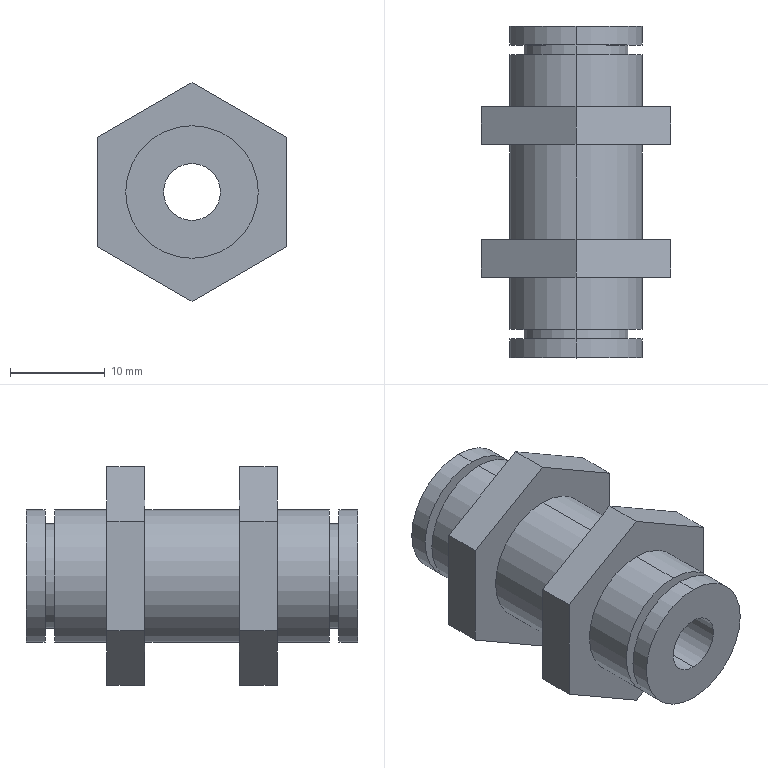Part | SolidWorks | features ICE 3, Revolution 1 | 2 solids | 38 faces | box 20 x 35 x 23.094 mm | volume 5820 mm3 | plane 22 | cylinder 16 | commonest cylinder face diameters 14 x10 11 x4 6 x2
STEP:
#1=CARTESIAN_POINT('',(0.,9.,-7.));
#2=VERTEX_POINT('',#1);
#3=CARTESIAN_POINT('',(0.,9.,7.));
#4=VERTEX_POINT('',#3);
#5=CARTESIAN_POINT('',(0.,9.,0.));
#6=DIRECTION('',(0.,1.,0.));
#7=DIRECTION('',(0.,0.,1.));
#8=AXIS2_PLACEMENT_3D('',#5,#6,#7);
#9=CIRCLE('',#8,7.);
#10=EDGE_CURVE('',#2,#4,#9,.T.);
#11=ORIENTED_EDGE('',*,*,#10,.T.);
#12=CARTESIAN_POINT('',(0.,5.,7.));
#13=VERTEX_POINT('',#12);
#14=CARTESIAN_POINT('',(0.,9.,7.));
#15=DIRECTION('',(0.,-1.,0.));
#16=VECTOR('',#15,1000.);
#17=LINE('',#14,#16);
#18=EDGE_CURVE('',#4,#13,#17,.T.);
#19=ORIENTED_EDGE('',*,*,#18,.T.);
#20=CARTESIAN_POINT('',(0.,5.,-7.));
#21=VERTEX_POINT('',#20);
#22=CARTESIAN_POINT('',(0.,5.,0.));
#23=DIRECTION('',(0.,1.,0.));
#24=DIRECTION('',(0.,0.,1.));
#25=AXIS2_PLACEMENT_3D('',#22,#23,#24);
#26=CIRCLE('',#25,7.);
#27=EDGE_CURVE('',#21,#13,#26,.T.);
#28=ORIENTED_EDGE('',*,*,#27,.F.);
#29=CARTESIAN_POINT('',(0.,9.,-7.));
#30=DIRECTION('',(0.,-1.,0.));
#31=VECTOR('',#30,1000.);
#32=LINE('',#29,#31);
#33=EDGE_CURVE('',#2,#21,#32,.T.);
#34=ORIENTED_EDGE('',*,*,#33,.F.);
#35=EDGE_LOOP('',(#11,#19,#28,#34));
#36=FACE_OUTER_BOUND('',#35,.T.);
#37=CARTESIAN_POINT('',(0.,9.,0.));
#38=DIRECTION('',(0.,-1.,0.));
#39=DIRECTION('',(0.,0.,-1.));
#40=AXIS2_PLACEMENT_3D('',#37,#38,#39);
#41=CYLINDRICAL_SURFACE('',#40,7.);
#42=ADVANCED_FACE('',(#36),#41,.F.);
#43=CARTESIAN_POINT('',(10.,9.,-5.774));
#44=VERTEX_POINT('',#43);
#45=CARTESIAN_POINT('',(0.,9.,-11.547));
#46=VERTEX_POINT('',#45);
#47=CARTESIAN_POINT('',(10.,9.,-5.774));
#48=DIRECTION('',(-0.866,0.,-0.5));
#49=VECTOR('',#48,1000.);
#50=LINE('',#47,#49);
#51=EDGE_CURVE('',#44,#46,#50,.T.);
#52=ORIENTED_EDGE('',*,*,#51,.T.);
#53=CARTESIAN_POINT('',(-10.,9.,-5.774));
#54=VERTEX_POINT('',#53);
#55=CARTESIAN_POINT('',(0.,9.,-11.547));
#56=DIRECTION('',(-0.866,0.,0.5));
#57=VECTOR('',#56,1000.);
#58=LINE('',#55,#57);
#59=EDGE_CURVE('',#46,#54,#58,.T.);
#60=ORIENTED_EDGE('',*,*,#59,.T.);
#61=CARTESIAN_POINT('',(-10.,9.,5.774));
#62=VERTEX_POINT('',#61);
#63=CARTESIAN_POINT('',(-10.,9.,-5.774));
#64=DIRECTION('',(0.,0.,1.));
#65=VECTOR('',#64,1000.);
#66=LINE('',#63,#65);
#67=EDGE_CURVE('',#54,#62,#66,.T.);
#68=ORIENTED_EDGE('',*,*,#67,.T.);
#69=CARTESIAN_POINT('',(0.,9.,11.547));
#70=VERTEX_POINT('',#69);
#71=CARTESIAN_POINT('',(-10.,9.,5.774));
#72=DIRECTION('',(0.866,0.,0.5));
#73=VECTOR('',#72,1000.);
#74=LINE('',#71,#73);
#75=EDGE_CURVE('',#62,#70,#74,.T.);
#76=ORIENTED_EDGE('',*,*,#75,.T.);
#77=CARTESIAN_POINT('',(10.,9.,5.774));
#78=VERTEX_POINT('',#77);
#79=CARTESIAN_POINT('',(0.,9.,11.547));
#80=DIRECTION('',(0.866,0.,-0.5));
#81=VECTOR('',#80,1000.);
#82=LINE('',#79,#81);
#83=EDGE_CURVE('',#70,#78,#82,.T.);
#84=ORIENTED_EDGE('',*,*,#83,.T.);
#85=CARTESIAN_POINT('',(10.,9.,5.774));
#86=DIRECTION('',(0.,0.,-1.));
#87=VECTOR('',#86,1000.);
#88=LINE('',#85,#87);
#89=EDGE_CURVE('',#78,#44,#88,.T.);
#90=ORIENTED_EDGE('',*,*,#89,.T.);
#91=EDGE_LOOP('',(#52,#60,#68,#76,#84,#90));
#92=FACE_OUTER_BOUND('',#91,.T.);
#93=ORIENTED_EDGE('',*,*,#10,.F.);
#94=CARTESIAN_POINT('',(0.,9.,0.));
#95=DIRECTION('',(0.,1.,0.));
#96=DIRECTION('',(0.,0.,1.));
#97=AXIS2_PLACEMENT_3D('',#94,#95,#96);
#98=CIRCLE('',#97,7.);
#99=EDGE_CURVE('',#4,#2,#98,.T.);
#100=ORIENTED_EDGE('',*,*,#99,.F.);
#101=EDGE_LOOP('',(#93,#100));
#102=FACE_BOUND('',#101,.T.);
#103=CARTESIAN_POINT('',(0.,9.,0.));
#104=DIRECTION('',(0.,1.,0.));
#105=DIRECTION('',(0.,0.,1.));
#106=AXIS2_PLACEMENT_3D('',#103,#104,#105);
#107=PLANE('',#106);
#108=ADVANCED_FACE('',(#92,#102),#107,.T.);
#109=CARTESIAN_POINT('',(10.,5.,-5.774));
#110=VERTEX_POINT('',#109);
#111=CARTESIAN_POINT('',(0.,5.,-11.547));
#112=VERTEX_POINT('',#111);
#113=CARTESIAN_POINT('',(10.,5.,-5.774));
#114=DIRECTION('',(-0.866,0.,-0.5));
#115=VECTOR('',#114,1000.);
#116=LINE('',#113,#115);
#117=EDGE_CURVE('',#110,#112,#116,.T.);
#118=ORIENTED_EDGE('',*,*,#117,.F.);
#119=CARTESIAN_POINT('',(10.,5.,5.774));
#120=VERTEX_POINT('',#119);
#121=CARTESIAN_POINT('',(10.,5.,5.774));
#122=DIRECTION('',(0.,0.,-1.));
#123=VECTOR('',#122,1000.);
#124=LINE('',#121,#123);
#125=EDGE_CURVE('',#120,#110,#124,.T.);
#126=ORIENTED_EDGE('',*,*,#125,.F.);
#127=CARTESIAN_POINT('',(0.,5.,11.547));
#128=VERTEX_POINT('',#127);
#129=CARTESIAN_POINT('',(0.,5.,11.547));
#130=DIRECTION('',(0.866,0.,-0.5));
#131=VECTOR('',#130,1000.);
#132=LINE('',#129,#131);
#133=EDGE_CURVE('',#128,#120,#132,.T.);
#134=ORIENTED_EDGE('',*,*,#133,.F.);
#135=CARTESIAN_POINT('',(-10.,5.,5.774));
#136=VERTEX_POINT('',#135);
#137=CARTESIAN_POINT('',(-10.,5.,5.774));
#138=DIRECTION('',(0.866,0.,0.5));
#139=VECTOR('',#138,1000.);
#140=LINE('',#137,#139);
#141=EDGE_CURVE('',#136,#128,#140,.T.);
#142=ORIENTED_EDGE('',*,*,#141,.F.);
#143=CARTESIAN_POINT('',(-10.,5.,-5.774));
#144=VERTEX_POINT('',#143);
#145=CARTESIAN_POINT('',(-10.,5.,-5.774));
#146=DIRECTION('',(0.,0.,1.));
#147=VECTOR('',#146,1000.);
#148=LINE('',#145,#147);
#149=EDGE_CURVE('',#144,#136,#148,.T.);
#150=ORIENTED_EDGE('',*,*,#149,.F.);
#151=CARTESIAN_POINT('',(0.,5.,-11.547));
#152=DIRECTION('',(-0.866,0.,0.5));
#153=VECTOR('',#152,1000.);
#154=LINE('',#151,#153);
#155=EDGE_CURVE('',#112,#144,#154,.T.);
#156=ORIENTED_EDGE('',*,*,#155,.F.);
#157=EDGE_LOOP('',(#118,#126,#134,#142,#150,#156));
#158=FACE_OUTER_BOUND('',#157,.T.);
#159=ORIENTED_EDGE('',*,*,#27,.T.);
#160=CARTESIAN_POINT('',(0.,5.,0.));
#161=DIRECTION('',(0.,1.,0.));
#162=DIRECTION('',(0.,0.,1.));
#163=AXIS2_PLACEMENT_3D('',#160,#161,#162);
#164=CIRCLE('',#163,7.);
#165=EDGE_CURVE('',#13,#21,#164,.T.);
#166=ORIENTED_EDGE('',*,*,#165,.T.);
#167=EDGE_LOOP('',(#159,#166));
#168=FACE_BOUND('',#167,.T.);
#169=CARTESIAN_POINT('',(0.,5.,0.));
#170=DIRECTION('',(0.,1.,0.));
#171=DIRECTION('',(0.,0.,1.));
#172=AXIS2_PLACEMENT_3D('',#169,#170,#171);
#173=PLANE('',#172);
#174=ADVANCED_FACE('',(#158,#168),#173,.F.);
#175=ORIENTED_EDGE('',*,*,#117,.T.);
#176=CARTESIAN_POINT('',(0.,9.,-11.547));
#177=DIRECTION('',(0.,-1.,0.));
#178=VECTOR('',#177,1000.);
#179=LINE('',#176,#178);
#180=EDGE_CURVE('',#46,#112,#179,.T.);
#181=ORIENTED_EDGE('',*,*,#180,.F.);
#182=ORIENTED_EDGE('',*,*,#51,.F.);
#183=CARTESIAN_POINT('',(10.,9.,-5.774));
#184=DIRECTION('',(0.,-1.,0.));
#185=VECTOR('',#184,1000.);
#186=LINE('',#183,#185);
#187=EDGE_CURVE('',#44,#110,#186,.T.);
#188=ORIENTED_EDGE('',*,*,#187,.T.);
#189=EDGE_LOOP('',(#175,#181,#182,#188));
#190=FACE_OUTER_BOUND('',#189,.T.);
#191=CARTESIAN_POINT('',(10.,9.,-5.774));
#192=DIRECTION('',(-0.5,0.,0.866));
#193=DIRECTION('',(0.866,0.,0.5));
#194=AXIS2_PLACEMENT_3D('',#191,#192,#193);
#195=PLANE('',#194);
#196=ADVANCED_FACE('',(#190),#195,.F.);
#197=ORIENTED_EDGE('',*,*,#155,.T.);
#198=CARTESIAN_POINT('',(-10.,9.,-5.774));
#199=DIRECTION('',(0.,-1.,0.));
#200=VECTOR('',#199,1000.);
#201=LINE('',#198,#200);
#202=EDGE_CURVE('',#54,#144,#201,.T.);
#203=ORIENTED_EDGE('',*,*,#202,.F.);
#204=ORIENTED_EDGE('',*,*,#59,.F.);
#205=ORIENTED_EDGE('',*,*,#180,.T.);
#206=EDGE_LOOP('',(#197,#203,#204,#205));
#207=FACE_OUTER_BOUND('',#206,.T.);
#208=CARTESIAN_POINT('',(0.,9.,-11.547));
#209=DIRECTION('',(0.5,0.,0.866));
#210=DIRECTION('',(0.866,0.,-0.5));
#211=AXIS2_PLACEMENT_3D('',#208,#209,#210);
#212=PLANE('',#211);
#213=ADVANCED_FACE('',(#207),#212,.F.);
#214=ORIENTED_EDGE('',*,*,#149,.T.);
#215=CARTESIAN_POINT('',(-10.,9.,5.774));
#216=DIRECTION('',(0.,-1.,0.));
#217=VECTOR('',#216,1000.);
#218=LINE('',#215,#217);
#219=EDGE_CURVE('',#62,#136,#218,.T.);
#220=ORIENTED_EDGE('',*,*,#219,.F.);
#221=ORIENTED_EDGE('',*,*,#67,.F.);
#222=ORIENTED_EDGE('',*,*,#202,.T.);
#223=EDGE_LOOP('',(#214,#220,#221,#222));
#224=FACE_OUTER_BOUND('',#223,.T.);
#225=CARTESIAN_POINT('',(-10.,9.,-5.774));
#226=DIRECTION('',(1.,0.,0.));
#227=DIRECTION('',(0.,0.,-1.));
#228=AXIS2_PLACEMENT_3D('',#225,#226,#227);
#229=PLANE('',#228);
#230=ADVANCED_FACE('',(#224),#229,.F.);
#231=ORIENTED_EDGE('',*,*,#141,.T.);
#232=CARTESIAN_POINT('',(0.,9.,11.547));
#233=DIRECTION('',(0.,-1.,0.));
#234=VECTOR('',#233,1000.);
#235=LINE('',#232,#234);
#236=EDGE_CURVE('',#70,#128,#235,.T.);
#237=ORIENTED_EDGE('',*,*,#236,.F.);
#238=ORIENTED_EDGE('',*,*,#75,.F.);
#239=ORIENTED_EDGE('',*,*,#219,.T.);
#240=EDGE_LOOP('',(#231,#237,#238,#239));
#241=FACE_OUTER_BOUND('',#240,.T.);
#242=CARTESIAN_POINT('',(-10.,9.,5.774));
#243=DIRECTION('',(0.5,0.,-0.866));
#244=DIRECTION('',(-0.866,0.,-0.5));
#245=AXIS2_PLACEMENT_3D('',#242,#243,#244);
#246=PLANE('',#245);
#247=ADVANCED_FACE('',(#241),#246,.F.);
#248=ORIENTED_EDGE('',*,*,#133,.T.);
#249=CARTESIAN_POINT('',(10.,9.,5.774));
#250=DIRECTION('',(0.,-1.,0.));
#251=VECTOR('',#250,1000.);
#252=LINE('',#249,#251);
#253=EDGE_CURVE('',#78,#120,#252,.T.);
#254=ORIENTED_EDGE('',*,*,#253,.F.);
#255=ORIENTED_EDGE('',*,*,#83,.F.);
#256=ORIENTED_EDGE('',*,*,#236,.T.);
#257=EDGE_LOOP('',(#248,#254,#255,#256));
#258=FACE_OUTER_BOUND('',#257,.T.);
#259=CARTESIAN_POINT('',(0.,9.,11.547));
#260=DIRECTION('',(-0.5,0.,-0.866));
#261=DIRECTION('',(-0.866,0.,0.5));
#262=AXIS2_PLACEMENT_3D('',#259,#260,#261);
#263=PLANE('',#262);
#264=ADVANCED_FACE('',(#258),#263,.F.);
#265=ORIENTED_EDGE('',*,*,#125,.T.);
#266=ORIENTED_EDGE('',*,*,#187,.F.);
#267=ORIENTED_EDGE('',*,*,#89,.F.);
#268=ORIENTED_EDGE('',*,*,#253,.T.);
#269=EDGE_LOOP('',(#265,#266,#267,#268));
#270=FACE_OUTER_BOUND('',#269,.T.);
#271=CARTESIAN_POINT('',(10.,9.,5.774));
#272=DIRECTION('',(-1.,0.,0.));
#273=DIRECTION('',(0.,0.,1.));
#274=AXIS2_PLACEMENT_3D('',#271,#272,#273);
#275=PLANE('',#274);
#276=ADVANCED_FACE('',(#270),#275,.F.);
#277=ORIENTED_EDGE('',*,*,#18,.F.);
#278=ORIENTED_EDGE('',*,*,#99,.T.);
#279=ORIENTED_EDGE('',*,*,#33,.T.);
#280=ORIENTED_EDGE('',*,*,#165,.F.);
#281=EDGE_LOOP('',(#277,#278,#279,#280));
#282=FACE_OUTER_BOUND('',#281,.T.);
#283=CARTESIAN_POINT('',(0.,9.,0.));
#284=DIRECTION('',(0.,-1.,0.));
#285=DIRECTION('',(0.,0.,-1.));
#286=AXIS2_PLACEMENT_3D('',#283,#284,#285);
#287=CYLINDRICAL_SURFACE('',#286,7.);
#288=ADVANCED_FACE('',(#282),#287,.F.);
#289=CLOSED_SHELL('',(#42,#108,#174,#196,#213,#230,#247,#264,#276,#288));
#290=MANIFOLD_SOLID_BREP('',#289);
#291=CARTESIAN_POINT('',(0.,-17.5,-3.));
#292=VERTEX_POINT('',#291);
#293=CARTESIAN_POINT('',(0.,-17.5,3.));
#294=VERTEX_POINT('',#293);
#295=CARTESIAN_POINT('',(0.,-17.5,0.));
#296=DIRECTION('',(0.,1.,0.));
#297=DIRECTION('',(0.,0.,1.));
#298=AXIS2_PLACEMENT_3D('',#295,#296,#297);
#299=CIRCLE('',#298,3.);
#300=EDGE_CURVE('',#292,#294,#299,.T.);
#301=ORIENTED_EDGE('',*,*,#300,.F.);
#302=CARTESIAN_POINT('',(0.,17.5,-3.));
#303=VERTEX_POINT('',#302);
#304=CARTESIAN_POINT('',(0.,-17.5,-3.));
#305=DIRECTION('',(0.,1.,0.));
#306=VECTOR('',#305,1000.);
#307=LINE('',#304,#306);
#308=EDGE_CURVE('',#292,#303,#307,.T.);
#309=ORIENTED_EDGE('',*,*,#308,.T.);
#310=CARTESIAN_POINT('',(0.,17.5,3.));
#311=VERTEX_POINT('',#310);
#312=CARTESIAN_POINT('',(0.,17.5,0.));
#313=DIRECTION('',(0.,1.,0.));
#314=DIRECTION('',(0.,0.,1.));
#315=AXIS2_PLACEMENT_3D('',#312,#313,#314);
#316=CIRCLE('',#315,3.);
#317=EDGE_CURVE('',#303,#311,#316,.T.);
#318=ORIENTED_EDGE('',*,*,#317,.T.);
#319=CARTESIAN_POINT('',(0.,-17.5,3.));
#320=DIRECTION('',(0.,1.,0.));
#321=VECTOR('',#320,1000.);
#322=LINE('',#319,#321);
#323=EDGE_CURVE('',#294,#311,#322,.T.);
#324=ORIENTED_EDGE('',*,*,#323,.F.);
#325=EDGE_LOOP('',(#301,#309,#318,#324));
#326=FACE_OUTER_BOUND('',#325,.T.);
#327=CARTESIAN_POINT('',(0.,-17.5,0.));
#328=DIRECTION('',(0.,1.,0.));
#329=DIRECTION('',(0.,0.,1.));
#330=AXIS2_PLACEMENT_3D('',#327,#328,#329);
#331=CYLINDRICAL_SURFACE('',#330,3.);
#332=ADVANCED_FACE('',(#326),#331,.F.);
#333=CARTESIAN_POINT('',(0.,15.5,7.));
#334=VERTEX_POINT('',#333);
#335=CARTESIAN_POINT('',(0.,15.5,-7.));
#336=VERTEX_POINT('',#335);
#337=CARTESIAN_POINT('',(0.,15.5,0.));
#338=DIRECTION('',(0.,1.,0.));
#339=DIRECTION('',(0.,0.,1.));
#340=AXIS2_PLACEMENT_3D('',#337,#338,#339);
#341=CIRCLE('',#340,7.);
#342=EDGE_CURVE('',#334,#336,#341,.T.);
#343=ORIENTED_EDGE('',*,*,#342,.T.);
#344=CARTESIAN_POINT('',(0.,17.5,-7.));
#345=VERTEX_POINT('',#344);
#346=CARTESIAN_POINT('',(0.,17.5,-7.));
#347=DIRECTION('',(0.,1.,0.));
#348=VECTOR('',#347,1000.);
#349=LINE('',#346,#348);
#350=EDGE_CURVE('',#336,#345,#349,.T.);
#351=ORIENTED_EDGE('',*,*,#350,.T.);
#352=CARTESIAN_POINT('',(0.,17.5,7.));
#353=VERTEX_POINT('',#352);
#354=CARTESIAN_POINT('',(0.,17.5,0.));
#355=DIRECTION('',(0.,1.,0.));
#356=DIRECTION('',(0.,0.,1.));
#357=AXIS2_PLACEMENT_3D('',#354,#355,#356);
#358=CIRCLE('',#357,7.);
#359=EDGE_CURVE('',#353,#345,#358,.T.);
#360=ORIENTED_EDGE('',*,*,#359,.F.);
#361=CARTESIAN_POINT('',(0.,17.5,7.));
#362=DIRECTION('',(0.,1.,0.));
#363=VECTOR('',#362,1000.);
#364=LINE('',#361,#363);
#365=EDGE_CURVE('',#334,#353,#364,.T.);
#366=ORIENTED_EDGE('',*,*,#365,.F.);
#367=EDGE_LOOP('',(#343,#351,#360,#366));
#368=FACE_OUTER_BOUND('',#367,.T.);
#369=CARTESIAN_POINT('',(0.,17.5,0.));
#370=DIRECTION('',(0.,1.,0.));
#371=DIRECTION('',(0.,0.,1.));
#372=AXIS2_PLACEMENT_3D('',#369,#370,#371);
#373=CYLINDRICAL_SURFACE('',#372,7.);
#374=ADVANCED_FACE('',(#368),#373,.T.);
#375=CARTESIAN_POINT('',(0.,14.5,5.5));
#376=VERTEX_POINT('',#375);
#377=CARTESIAN_POINT('',(0.,14.5,-5.5));
#378=VERTEX_POINT('',#377);
#379=CARTESIAN_POINT('',(0.,14.5,0.));
#380=DIRECTION('',(0.,1.,0.));
#381=DIRECTION('',(0.,0.,1.));
#382=AXIS2_PLACEMENT_3D('',#379,#380,#381);
#383=CIRCLE('',#382,5.5);
#384=EDGE_CURVE('',#376,#378,#383,.T.);
#385=ORIENTED_EDGE('',*,*,#384,.T.);
#386=CARTESIAN_POINT('',(0.,15.5,-5.5));
#387=VERTEX_POINT('',#386);
#388=CARTESIAN_POINT('',(0.,17.5,-5.5));
#389=DIRECTION('',(0.,1.,0.));
#390=VECTOR('',#389,1000.);
#391=LINE('',#388,#390);
#392=EDGE_CURVE('',#378,#387,#391,.T.);
#393=ORIENTED_EDGE('',*,*,#392,.T.);
#394=CARTESIAN_POINT('',(0.,15.5,5.5));
#395=VERTEX_POINT('',#394);
#396=CARTESIAN_POINT('',(0.,15.5,0.));
#397=DIRECTION('',(0.,1.,0.));
#398=DIRECTION('',(0.,0.,1.));
#399=AXIS2_PLACEMENT_3D('',#396,#397,#398);
#400=CIRCLE('',#399,5.5);
#401=EDGE_CURVE('',#395,#387,#400,.T.);
#402=ORIENTED_EDGE('',*,*,#401,.F.);
#403=CARTESIAN_POINT('',(0.,17.5,5.5));
#404=DIRECTION('',(0.,1.,0.));
#405=VECTOR('',#404,1000.);
#406=LINE('',#403,#405);
#407=EDGE_CURVE('',#376,#395,#406,.T.);
#408=ORIENTED_EDGE('',*,*,#407,.F.);
#409=EDGE_LOOP('',(#385,#393,#402,#408));
#410=FACE_OUTER_BOUND('',#409,.T.);
#411=CARTESIAN_POINT('',(0.,17.5,0.));
#412=DIRECTION('',(0.,1.,0.));
#413=DIRECTION('',(0.,0.,1.));
#414=AXIS2_PLACEMENT_3D('',#411,#412,#413);
#415=CYLINDRICAL_SURFACE('',#414,5.5);
#416=ADVANCED_FACE('',(#410),#415,.T.);
#417=CARTESIAN_POINT('',(0.,-5.,-7.));
#418=VERTEX_POINT('',#417);
#419=CARTESIAN_POINT('',(0.,-5.,7.));
#420=VERTEX_POINT('',#419);
#421=CARTESIAN_POINT('',(0.,-5.,0.));
#422=DIRECTION('',(0.,-1.,0.));
#423=DIRECTION('',(0.,0.,1.));
#424=AXIS2_PLACEMENT_3D('',#421,#422,#423);
#425=CIRCLE('',#424,7.);
#426=EDGE_CURVE('',#418,#420,#425,.T.);
#427=ORIENTED_EDGE('',*,*,#426,.F.);
#428=CARTESIAN_POINT('',(0.,14.5,-7.));
#429=VERTEX_POINT('',#428);
#430=CARTESIAN_POINT('',(0.,17.5,-7.));
#431=DIRECTION('',(0.,1.,0.));
#432=VECTOR('',#431,1000.);
#433=LINE('',#430,#432);
#434=EDGE_CURVE('',#418,#429,#433,.T.);
#435=ORIENTED_EDGE('',*,*,#434,.T.);
#436=CARTESIAN_POINT('',(0.,14.5,7.));
#437=VERTEX_POINT('',#436);
#438=CARTESIAN_POINT('',(0.,14.5,0.));
#439=DIRECTION('',(0.,1.,0.));
#440=DIRECTION('',(0.,0.,1.));
#441=AXIS2_PLACEMENT_3D('',#438,#439,#440);
#442=CIRCLE('',#441,7.);
#443=EDGE_CURVE('',#437,#429,#442,.T.);
#444=ORIENTED_EDGE('',*,*,#443,.F.);
#445=CARTESIAN_POINT('',(0.,17.5,7.));
#446=DIRECTION('',(0.,1.,0.));
#447=VECTOR('',#446,1000.);
#448=LINE('',#445,#447);
#449=EDGE_CURVE('',#420,#437,#448,.T.);
#450=ORIENTED_EDGE('',*,*,#449,.F.);
#451=EDGE_LOOP('',(#427,#435,#444,#450));
#452=FACE_OUTER_BOUND('',#451,.T.);
#453=CARTESIAN_POINT('',(0.,17.5,0.));
#454=DIRECTION('',(0.,1.,0.));
#455=DIRECTION('',(0.,0.,1.));
#456=AXIS2_PLACEMENT_3D('',#453,#454,#455);
#457=CYLINDRICAL_SURFACE('',#456,7.);
#458=ADVANCED_FACE('',(#452),#457,.T.);
#459=CARTESIAN_POINT('',(0.,-15.5,5.5));
#460=VERTEX_POINT('',#459);
#461=CARTESIAN_POINT('',(0.,-15.5,-5.5));
#462=VERTEX_POINT('',#461);
#463=CARTESIAN_POINT('',(0.,-15.5,0.));
#464=DIRECTION('',(0.,1.,0.));
#465=DIRECTION('',(0.,0.,1.));
#466=AXIS2_PLACEMENT_3D('',#463,#464,#465);
#467=CIRCLE('',#466,5.5);
#468=EDGE_CURVE('',#460,#462,#467,.T.);
#469=ORIENTED_EDGE('',*,*,#468,.T.);
#470=CARTESIAN_POINT('',(0.,-14.5,-5.5));
#471=VERTEX_POINT('',#470);
#472=CARTESIAN_POINT('',(0.,17.5,-5.5));
#473=DIRECTION('',(0.,1.,0.));
#474=VECTOR('',#473,1000.);
#475=LINE('',#472,#474);
#476=EDGE_CURVE('',#462,#471,#475,.T.);
#477=ORIENTED_EDGE('',*,*,#476,.T.);
#478=CARTESIAN_POINT('',(0.,-14.5,5.5));
#479=VERTEX_POINT('',#478);
#480=CARTESIAN_POINT('',(0.,-14.5,0.));
#481=DIRECTION('',(0.,1.,0.));
#482=DIRECTION('',(0.,0.,1.));
#483=AXIS2_PLACEMENT_3D('',#480,#481,#482);
#484=CIRCLE('',#483,5.5);
#485=EDGE_CURVE('',#479,#471,#484,.T.);
#486=ORIENTED_EDGE('',*,*,#485,.F.);
#487=CARTESIAN_POINT('',(0.,17.5,5.5));
#488=DIRECTION('',(0.,1.,0.));
#489=VECTOR('',#488,1000.);
#490=LINE('',#487,#489);
#491=EDGE_CURVE('',#460,#479,#490,.T.);
#492=ORIENTED_EDGE('',*,*,#491,.F.);
#493=EDGE_LOOP('',(#469,#477,#486,#492));
#494=FACE_OUTER_BOUND('',#493,.T.);
#495=CARTESIAN_POINT('',(0.,17.5,0.));
#496=DIRECTION('',(0.,1.,0.));
#497=DIRECTION('',(0.,0.,1.));
#498=AXIS2_PLACEMENT_3D('',#495,#496,#497);
#499=CYLINDRICAL_SURFACE('',#498,5.5);
#500=ADVANCED_FACE('',(#494),#499,.T.);
#501=CARTESIAN_POINT('',(0.,-17.5,7.));
#502=VERTEX_POINT('',#501);
#503=CARTESIAN_POINT('',(0.,-17.5,-7.));
#504=VERTEX_POINT('',#503);
#505=CARTESIAN_POINT('',(0.,-17.5,0.));
#506=DIRECTION('',(0.,1.,0.));
#507=DIRECTION('',(0.,0.,1.));
#508=AXIS2_PLACEMENT_3D('',#505,#506,#507);
#509=CIRCLE('',#508,7.);
#510=EDGE_CURVE('',#502,#504,#509,.T.);
#511=ORIENTED_EDGE('',*,*,#510,.T.);
#512=CARTESIAN_POINT('',(0.,-15.5,-7.));
#513=VERTEX_POINT('',#512);
#514=CARTESIAN_POINT('',(0.,17.5,-7.));
#515=DIRECTION('',(0.,1.,0.));
#516=VECTOR('',#515,1000.);
#517=LINE('',#514,#516);
#518=EDGE_CURVE('',#504,#513,#517,.T.);
#519=ORIENTED_EDGE('',*,*,#518,.T.);
#520=CARTESIAN_POINT('',(0.,-15.5,7.));
#521=VERTEX_POINT('',#520);
#522=CARTESIAN_POINT('',(0.,-15.5,0.));
#523=DIRECTION('',(0.,1.,0.));
#524=DIRECTION('',(0.,0.,1.));
#525=AXIS2_PLACEMENT_3D('',#522,#523,#524);
#526=CIRCLE('',#525,7.);
#527=EDGE_CURVE('',#521,#513,#526,.T.);
#528=ORIENTED_EDGE('',*,*,#527,.F.);
#529=CARTESIAN_POINT('',(0.,17.5,7.));
#530=DIRECTION('',(0.,1.,0.));
#531=VECTOR('',#530,1000.);
#532=LINE('',#529,#531);
#533=EDGE_CURVE('',#502,#521,#532,.T.);
#534=ORIENTED_EDGE('',*,*,#533,.F.);
#535=EDGE_LOOP('',(#511,#519,#528,#534));
#536=FACE_OUTER_BOUND('',#535,.T.);
#537=CARTESIAN_POINT('',(0.,17.5,0.));
#538=DIRECTION('',(0.,1.,0.));
#539=DIRECTION('',(0.,0.,1.));
#540=AXIS2_PLACEMENT_3D('',#537,#538,#539);
#541=CYLINDRICAL_SURFACE('',#540,7.);
#542=ADVANCED_FACE('',(#536),#541,.T.);
#543=CARTESIAN_POINT('',(0.,-14.5,7.));
#544=VERTEX_POINT('',#543);
#545=CARTESIAN_POINT('',(0.,-14.5,-7.));
#546=VERTEX_POINT('',#545);
#547=CARTESIAN_POINT('',(0.,-14.5,0.));
#548=DIRECTION('',(0.,1.,0.));
#549=DIRECTION('',(0.,0.,1.));
#550=AXIS2_PLACEMENT_3D('',#547,#548,#549);
#551=CIRCLE('',#550,7.);
#552=EDGE_CURVE('',#544,#546,#551,.T.);
#553=ORIENTED_EDGE('',*,*,#552,.T.);
#554=CARTESIAN_POINT('',(0.,-9.,-7.));
#555=VERTEX_POINT('',#554);
#556=CARTESIAN_POINT('',(0.,17.5,-7.));
#557=DIRECTION('',(0.,1.,0.));
#558=VECTOR('',#557,1000.);
#559=LINE('',#556,#558);
#560=EDGE_CURVE('',#546,#555,#559,.T.);
#561=ORIENTED_EDGE('',*,*,#560,.T.);
#562=CARTESIAN_POINT('',(0.,-9.,7.));
#563=VERTEX_POINT('',#562);
#564=CARTESIAN_POINT('',(0.,-9.,0.));
#565=DIRECTION('',(0.,1.,0.));
#566=DIRECTION('',(0.,0.,1.));
#567=AXIS2_PLACEMENT_3D('',#564,#565,#566);
#568=CIRCLE('',#567,7.);
#569=EDGE_CURVE('',#563,#555,#568,.T.);
#570=ORIENTED_EDGE('',*,*,#569,.F.);
#571=CARTESIAN_POINT('',(0.,17.5,7.));
#572=DIRECTION('',(0.,1.,0.));
#573=VECTOR('',#572,1000.);
#574=LINE('',#571,#573);
#575=EDGE_CURVE('',#544,#563,#574,.T.);
#576=ORIENTED_EDGE('',*,*,#575,.F.);
#577=EDGE_LOOP('',(#553,#561,#570,#576));
#578=FACE_OUTER_BOUND('',#577,.T.);
#579=CARTESIAN_POINT('',(0.,17.5,0.));
#580=DIRECTION('',(0.,1.,0.));
#581=DIRECTION('',(0.,0.,1.));
#582=AXIS2_PLACEMENT_3D('',#579,#580,#581);
#583=CYLINDRICAL_SURFACE('',#582,7.);
#584=ADVANCED_FACE('',(#578),#583,.T.);
#585=ORIENTED_EDGE('',*,*,#560,.F.);
#586=CARTESIAN_POINT('',(0.,-14.5,0.));
#587=DIRECTION('',(0.,1.,0.));
#588=DIRECTION('',(0.,0.,1.));
#589=AXIS2_PLACEMENT_3D('',#586,#587,#588);
#590=CIRCLE('',#589,7.);
#591=EDGE_CURVE('',#546,#544,#590,.T.);
#592=ORIENTED_EDGE('',*,*,#591,.T.);
#593=ORIENTED_EDGE('',*,*,#575,.T.);
#594=CARTESIAN_POINT('',(0.,-9.,0.));
#595=DIRECTION('',(0.,1.,0.));
#596=DIRECTION('',(0.,0.,1.));
#597=AXIS2_PLACEMENT_3D('',#594,#595,#596);
#598=CIRCLE('',#597,7.);
#599=EDGE_CURVE('',#555,#563,#598,.T.);
#600=ORIENTED_EDGE('',*,*,#599,.F.);
#601=EDGE_LOOP('',(#585,#592,#593,#600));
#602=FACE_OUTER_BOUND('',#601,.T.);
#603=CARTESIAN_POINT('',(0.,17.5,0.));
#604=DIRECTION('',(0.,1.,0.));
#605=DIRECTION('',(0.,0.,1.));
#606=AXIS2_PLACEMENT_3D('',#603,#604,#605);
#607=CYLINDRICAL_SURFACE('',#606,7.);
#608=ADVANCED_FACE('',(#602),#607,.T.);
#609=CARTESIAN_POINT('',(0.,-17.5,0.));
#610=DIRECTION('',(0.,1.,0.));
#611=DIRECTION('',(0.,0.,1.));
#612=AXIS2_PLACEMENT_3D('',#609,#610,#611);
#613=CIRCLE('',#612,3.);
#614=EDGE_CURVE('',#294,#292,#613,.T.);
#615=ORIENTED_EDGE('',*,*,#614,.T.);
#616=ORIENTED_EDGE('',*,*,#300,.T.);
#617=EDGE_LOOP('',(#615,#616));
#618=FACE_BOUND('',#617,.T.);
#619=ORIENTED_EDGE('',*,*,#510,.F.);
#620=CARTESIAN_POINT('',(0.,-17.5,0.));
#621=DIRECTION('',(0.,1.,0.));
#622=DIRECTION('',(0.,0.,1.));
#623=AXIS2_PLACEMENT_3D('',#620,#621,#622);
#624=CIRCLE('',#623,7.);
#625=EDGE_CURVE('',#504,#502,#624,.T.);
#626=ORIENTED_EDGE('',*,*,#625,.F.);
#627=EDGE_LOOP('',(#619,#626));
#628=FACE_OUTER_BOUND('',#627,.T.);
#629=CARTESIAN_POINT('',(0.,-17.5,0.));
#630=DIRECTION('',(0.,-1.,0.));
#631=DIRECTION('',(0.,0.,-1.));
#632=AXIS2_PLACEMENT_3D('',#629,#630,#631);
#633=PLANE('',#632);
#634=ADVANCED_FACE('',(#618,#628),#633,.T.);
#635=ORIENTED_EDGE('',*,*,#518,.F.);
#636=ORIENTED_EDGE('',*,*,#625,.T.);
#637=ORIENTED_EDGE('',*,*,#533,.T.);
#638=CARTESIAN_POINT('',(0.,-15.5,0.));
#639=DIRECTION('',(0.,1.,0.));
#640=DIRECTION('',(0.,0.,1.));
#641=AXIS2_PLACEMENT_3D('',#638,#639,#640);
#642=CIRCLE('',#641,7.);
#643=EDGE_CURVE('',#513,#521,#642,.T.);
#644=ORIENTED_EDGE('',*,*,#643,.F.);
#645=EDGE_LOOP('',(#635,#636,#637,#644));
#646=FACE_OUTER_BOUND('',#645,.T.);
#647=CARTESIAN_POINT('',(0.,17.5,0.));
#648=DIRECTION('',(0.,1.,0.));
#649=DIRECTION('',(0.,0.,1.));
#650=AXIS2_PLACEMENT_3D('',#647,#648,#649);
#651=CYLINDRICAL_SURFACE('',#650,7.);
#652=ADVANCED_FACE('',(#646),#651,.T.);
#653=ORIENTED_EDGE('',*,*,#527,.T.);
#654=ORIENTED_EDGE('',*,*,#643,.T.);
#655=EDGE_LOOP('',(#653,#654));
#656=FACE_OUTER_BOUND('',#655,.T.);
#657=ORIENTED_EDGE('',*,*,#468,.F.);
#658=CARTESIAN_POINT('',(0.,-15.5,0.));
#659=DIRECTION('',(0.,1.,0.));
#660=DIRECTION('',(0.,0.,1.));
#661=AXIS2_PLACEMENT_3D('',#658,#659,#660);
#662=CIRCLE('',#661,5.5);
#663=EDGE_CURVE('',#462,#460,#662,.T.);
#664=ORIENTED_EDGE('',*,*,#663,.F.);
#665=EDGE_LOOP('',(#657,#664));
#666=FACE_BOUND('',#665,.T.);
#667=CARTESIAN_POINT('',(-7.,-15.5,0.));
#668=DIRECTION('',(0.,1.,0.));
#669=DIRECTION('',(0.,0.,1.));
#670=AXIS2_PLACEMENT_3D('',#667,#668,#669);
#671=PLANE('',#670);
#672=ADVANCED_FACE('',(#656,#666),#671,.T.);
#673=ORIENTED_EDGE('',*,*,#476,.F.);
#674=ORIENTED_EDGE('',*,*,#663,.T.);
#675=ORIENTED_EDGE('',*,*,#491,.T.);
#676=CARTESIAN_POINT('',(0.,-14.5,0.));
#677=DIRECTION('',(0.,1.,0.));
#678=DIRECTION('',(0.,0.,1.));
#679=AXIS2_PLACEMENT_3D('',#676,#677,#678);
#680=CIRCLE('',#679,5.5);
#681=EDGE_CURVE('',#471,#479,#680,.T.);
#682=ORIENTED_EDGE('',*,*,#681,.F.);
#683=EDGE_LOOP('',(#673,#674,#675,#682));
#684=FACE_OUTER_BOUND('',#683,.T.);
#685=CARTESIAN_POINT('',(0.,17.5,0.));
#686=DIRECTION('',(0.,1.,0.));
#687=DIRECTION('',(0.,0.,1.));
#688=AXIS2_PLACEMENT_3D('',#685,#686,#687);
#689=CYLINDRICAL_SURFACE('',#688,5.5);
#690=ADVANCED_FACE('',(#684),#689,.T.);
#691=ORIENTED_EDGE('',*,*,#485,.T.);
#692=ORIENTED_EDGE('',*,*,#681,.T.);
#693=EDGE_LOOP('',(#691,#692));
#694=FACE_BOUND('',#693,.T.);
#695=ORIENTED_EDGE('',*,*,#552,.F.);
#696=ORIENTED_EDGE('',*,*,#591,.F.);
#697=EDGE_LOOP('',(#695,#696));
#698=FACE_OUTER_BOUND('',#697,.T.);
#699=CARTESIAN_POINT('',(-5.5,-14.5,0.));
#700=DIRECTION('',(0.,-1.,0.));
#701=DIRECTION('',(0.,0.,-1.));
#702=AXIS2_PLACEMENT_3D('',#699,#700,#701);
#703=PLANE('',#702);
#704=ADVANCED_FACE('',(#694,#698),#703,.T.);
#705=ORIENTED_EDGE('',*,*,#434,.F.);
#706=CARTESIAN_POINT('',(0.,-5.,0.));
#707=DIRECTION('',(0.,-1.,0.));
#708=DIRECTION('',(0.,0.,1.));
#709=AXIS2_PLACEMENT_3D('',#706,#707,#708);
#710=CIRCLE('',#709,7.);
#711=EDGE_CURVE('',#420,#418,#710,.T.);
#712=ORIENTED_EDGE('',*,*,#711,.F.);
#713=ORIENTED_EDGE('',*,*,#449,.T.);
#714=CARTESIAN_POINT('',(0.,14.5,0.));
#715=DIRECTION('',(0.,1.,0.));
#716=DIRECTION('',(0.,0.,1.));
#717=AXIS2_PLACEMENT_3D('',#714,#715,#716);
#718=CIRCLE('',#717,7.);
#719=EDGE_CURVE('',#429,#437,#718,.T.);
#720=ORIENTED_EDGE('',*,*,#719,.F.);
#721=EDGE_LOOP('',(#705,#712,#713,#720));
#722=FACE_OUTER_BOUND('',#721,.T.);
#723=CARTESIAN_POINT('',(0.,17.5,0.));
#724=DIRECTION('',(0.,1.,0.));
#725=DIRECTION('',(0.,0.,1.));
#726=AXIS2_PLACEMENT_3D('',#723,#724,#725);
#727=CYLINDRICAL_SURFACE('',#726,7.);
#728=ADVANCED_FACE('',(#722),#727,.T.);
#729=ORIENTED_EDGE('',*,*,#443,.T.);
#730=ORIENTED_EDGE('',*,*,#719,.T.);
#731=EDGE_LOOP('',(#729,#730));
#732=FACE_OUTER_BOUND('',#731,.T.);
#733=ORIENTED_EDGE('',*,*,#384,.F.);
#734=CARTESIAN_POINT('',(0.,14.5,0.));
#735=DIRECTION('',(0.,1.,0.));
#736=DIRECTION('',(0.,0.,1.));
#737=AXIS2_PLACEMENT_3D('',#734,#735,#736);
#738=CIRCLE('',#737,5.5);
#739=EDGE_CURVE('',#378,#376,#738,.T.);
#740=ORIENTED_EDGE('',*,*,#739,.F.);
#741=EDGE_LOOP('',(#733,#740));
#742=FACE_BOUND('',#741,.T.);
#743=CARTESIAN_POINT('',(-5.5,14.5,0.));
#744=DIRECTION('',(0.,1.,0.));
#745=DIRECTION('',(0.,0.,1.));
#746=AXIS2_PLACEMENT_3D('',#743,#744,#745);
#747=PLANE('',#746);
#748=ADVANCED_FACE('',(#732,#742),#747,.T.);
#749=ORIENTED_EDGE('',*,*,#392,.F.);
#750=ORIENTED_EDGE('',*,*,#739,.T.);
#751=ORIENTED_EDGE('',*,*,#407,.T.);
#752=CARTESIAN_POINT('',(0.,15.5,0.));
#753=DIRECTION('',(0.,1.,0.));
#754=DIRECTION('',(0.,0.,1.));
#755=AXIS2_PLACEMENT_3D('',#752,#753,#754);
#756=CIRCLE('',#755,5.5);
#757=EDGE_CURVE('',#387,#395,#756,.T.);
#758=ORIENTED_EDGE('',*,*,#757,.F.);
#759=EDGE_LOOP('',(#749,#750,#751,#758));
#760=FACE_OUTER_BOUND('',#759,.T.);
#761=CARTESIAN_POINT('',(0.,17.5,0.));
#762=DIRECTION('',(0.,1.,0.));
#763=DIRECTION('',(0.,0.,1.));
#764=AXIS2_PLACEMENT_3D('',#761,#762,#763);
#765=CYLINDRICAL_SURFACE('',#764,5.5);
#766=ADVANCED_FACE('',(#760),#765,.T.);
#767=ORIENTED_EDGE('',*,*,#401,.T.);
#768=ORIENTED_EDGE('',*,*,#757,.T.);
#769=EDGE_LOOP('',(#767,#768));
#770=FACE_BOUND('',#769,.T.);
#771=ORIENTED_EDGE('',*,*,#342,.F.);
#772=CARTESIAN_POINT('',(0.,15.5,0.));
#773=DIRECTION('',(0.,1.,0.));
#774=DIRECTION('',(0.,0.,1.));
#775=AXIS2_PLACEMENT_3D('',#772,#773,#774);
#776=CIRCLE('',#775,7.);
#777=EDGE_CURVE('',#336,#334,#776,.T.);
#778=ORIENTED_EDGE('',*,*,#777,.F.);
#779=EDGE_LOOP('',(#771,#778));
#780=FACE_OUTER_BOUND('',#779,.T.);
#781=CARTESIAN_POINT('',(-7.,15.5,0.));
#782=DIRECTION('',(0.,-1.,0.));
#783=DIRECTION('',(0.,0.,-1.));
#784=AXIS2_PLACEMENT_3D('',#781,#782,#783);
#785=PLANE('',#784);
#786=ADVANCED_FACE('',(#770,#780),#785,.T.);
#787=ORIENTED_EDGE('',*,*,#350,.F.);
#788=ORIENTED_EDGE('',*,*,#777,.T.);
#789=ORIENTED_EDGE('',*,*,#365,.T.);
#790=CARTESIAN_POINT('',(0.,17.5,0.));
#791=DIRECTION('',(0.,1.,0.));
#792=DIRECTION('',(0.,0.,1.));
#793=AXIS2_PLACEMENT_3D('',#790,#791,#792);
#794=CIRCLE('',#793,7.);
#795=EDGE_CURVE('',#345,#353,#794,.T.);
#796=ORIENTED_EDGE('',*,*,#795,.F.);
#797=EDGE_LOOP('',(#787,#788,#789,#796));
#798=FACE_OUTER_BOUND('',#797,.T.);
#799=CARTESIAN_POINT('',(0.,17.5,0.));
#800=DIRECTION('',(0.,1.,0.));
#801=DIRECTION('',(0.,0.,1.));
#802=AXIS2_PLACEMENT_3D('',#799,#800,#801);
#803=CYLINDRICAL_SURFACE('',#802,7.);
#804=ADVANCED_FACE('',(#798),#803,.T.);
#805=CARTESIAN_POINT('',(0.,17.5,0.));
#806=DIRECTION('',(0.,1.,0.));
#807=DIRECTION('',(0.,0.,1.));
#808=AXIS2_PLACEMENT_3D('',#805,#806,#807);
#809=CIRCLE('',#808,3.);
#810=EDGE_CURVE('',#311,#303,#809,.T.);
#811=ORIENTED_EDGE('',*,*,#810,.F.);
#812=ORIENTED_EDGE('',*,*,#317,.F.);
#813=EDGE_LOOP('',(#811,#812));
#814=FACE_BOUND('',#813,.T.);
#815=ORIENTED_EDGE('',*,*,#359,.T.);
#816=ORIENTED_EDGE('',*,*,#795,.T.);
#817=EDGE_LOOP('',(#815,#816));
#818=FACE_OUTER_BOUND('',#817,.T.);
#819=CARTESIAN_POINT('',(0.,17.5,0.));
#820=DIRECTION('',(0.,1.,0.));
#821=DIRECTION('',(0.,0.,1.));
#822=AXIS2_PLACEMENT_3D('',#819,#820,#821);
#823=PLANE('',#822);
#824=ADVANCED_FACE('',(#814,#818),#823,.T.);
#825=ORIENTED_EDGE('',*,*,#308,.F.);
#826=ORIENTED_EDGE('',*,*,#614,.F.);
#827=ORIENTED_EDGE('',*,*,#323,.T.);
#828=ORIENTED_EDGE('',*,*,#810,.T.);
#829=EDGE_LOOP('',(#825,#826,#827,#828));
#830=FACE_OUTER_BOUND('',#829,.T.);
#831=CARTESIAN_POINT('',(0.,-17.5,0.));
#832=DIRECTION('',(0.,1.,0.));
#833=DIRECTION('',(0.,0.,1.));
#834=AXIS2_PLACEMENT_3D('',#831,#832,#833);
#835=CYLINDRICAL_SURFACE('',#834,3.);
#836=ADVANCED_FACE('',(#830),#835,.F.);
#837=CARTESIAN_POINT('',(10.,-5.,-5.774));
#838=VERTEX_POINT('',#837);
#839=CARTESIAN_POINT('',(0.,-5.,-11.547));
#840=VERTEX_POINT('',#839);
#841=CARTESIAN_POINT('',(10.,-5.,-5.774));
#842=DIRECTION('',(-0.866,0.,-0.5));
#843=VECTOR('',#842,1000.);
#844=LINE('',#841,#843);
#845=EDGE_CURVE('',#838,#840,#844,.T.);
#846=ORIENTED_EDGE('',*,*,#845,.F.);
#847=CARTESIAN_POINT('',(10.,-9.,-5.774));
#848=VERTEX_POINT('',#847);
#849=CARTESIAN_POINT('',(10.,-9.,-5.774));
#850=DIRECTION('',(0.,1.,0.));
#851=VECTOR('',#850,1000.);
#852=LINE('',#849,#851);
#853=EDGE_CURVE('',#848,#838,#852,.T.);
#854=ORIENTED_EDGE('',*,*,#853,.F.);
#855=CARTESIAN_POINT('',(0.,-9.,-11.547));
#856=VERTEX_POINT('',#855);
#857=CARTESIAN_POINT('',(10.,-9.,-5.774));
#858=DIRECTION('',(-0.866,0.,-0.5));
#859=VECTOR('',#858,1000.);
#860=LINE('',#857,#859);
#861=EDGE_CURVE('',#848,#856,#860,.T.);
#862=ORIENTED_EDGE('',*,*,#861,.T.);
#863=CARTESIAN_POINT('',(0.,-9.,-11.547));
#864=DIRECTION('',(0.,1.,0.));
#865=VECTOR('',#864,1000.);
#866=LINE('',#863,#865);
#867=EDGE_CURVE('',#856,#840,#866,.T.);
#868=ORIENTED_EDGE('',*,*,#867,.T.);
#869=EDGE_LOOP('',(#846,#854,#862,#868));
#870=FACE_OUTER_BOUND('',#869,.T.);
#871=CARTESIAN_POINT('',(10.,-9.,-5.774));
#872=DIRECTION('',(0.5,0.,-0.866));
#873=DIRECTION('',(-0.866,0.,-0.5));
#874=AXIS2_PLACEMENT_3D('',#871,#872,#873);
#875=PLANE('',#874);
#876=ADVANCED_FACE('',(#870),#875,.T.);
#877=CARTESIAN_POINT('',(10.,-5.,5.774));
#878=VERTEX_POINT('',#877);
#879=CARTESIAN_POINT('',(10.,-5.,5.774));
#880=DIRECTION('',(0.,0.,-1.));
#881=VECTOR('',#880,1000.);
#882=LINE('',#879,#881);
#883=EDGE_CURVE('',#878,#838,#882,.T.);
#884=ORIENTED_EDGE('',*,*,#883,.F.);
#885=CARTESIAN_POINT('',(10.,-9.,5.774));
#886=VERTEX_POINT('',#885);
#887=CARTESIAN_POINT('',(10.,-9.,5.774));
#888=DIRECTION('',(0.,1.,0.));
#889=VECTOR('',#888,1000.);
#890=LINE('',#887,#889);
#891=EDGE_CURVE('',#886,#878,#890,.T.);
#892=ORIENTED_EDGE('',*,*,#891,.F.);
#893=CARTESIAN_POINT('',(10.,-9.,5.774));
#894=DIRECTION('',(0.,0.,-1.));
#895=VECTOR('',#894,1000.);
#896=LINE('',#893,#895);
#897=EDGE_CURVE('',#886,#848,#896,.T.);
#898=ORIENTED_EDGE('',*,*,#897,.T.);
#899=ORIENTED_EDGE('',*,*,#853,.T.);
#900=EDGE_LOOP('',(#884,#892,#898,#899));
#901=FACE_OUTER_BOUND('',#900,.T.);
#902=CARTESIAN_POINT('',(10.,-9.,5.774));
#903=DIRECTION('',(1.,0.,0.));
#904=DIRECTION('',(0.,0.,-1.));
#905=AXIS2_PLACEMENT_3D('',#902,#903,#904);
#906=PLANE('',#905);
#907=ADVANCED_FACE('',(#901),#906,.T.);
#908=CARTESIAN_POINT('',(0.,-5.,11.547));
#909=VERTEX_POINT('',#908);
#910=CARTESIAN_POINT('',(0.,-5.,11.547));
#911=DIRECTION('',(0.866,0.,-0.5));
#912=VECTOR('',#911,1000.);
#913=LINE('',#910,#912);
#914=EDGE_CURVE('',#909,#878,#913,.T.);
#915=ORIENTED_EDGE('',*,*,#914,.F.);
#916=CARTESIAN_POINT('',(0.,-9.,11.547));
#917=VERTEX_POINT('',#916);
#918=CARTESIAN_POINT('',(0.,-9.,11.547));
#919=DIRECTION('',(0.,1.,0.));
#920=VECTOR('',#919,1000.);
#921=LINE('',#918,#920);
#922=EDGE_CURVE('',#917,#909,#921,.T.);
#923=ORIENTED_EDGE('',*,*,#922,.F.);
#924=CARTESIAN_POINT('',(0.,-9.,11.547));
#925=DIRECTION('',(0.866,0.,-0.5));
#926=VECTOR('',#925,1000.);
#927=LINE('',#924,#926);
#928=EDGE_CURVE('',#917,#886,#927,.T.);
#929=ORIENTED_EDGE('',*,*,#928,.T.);
#930=ORIENTED_EDGE('',*,*,#891,.T.);
#931=EDGE_LOOP('',(#915,#923,#929,#930));
#932=FACE_OUTER_BOUND('',#931,.T.);
#933=CARTESIAN_POINT('',(0.,-9.,11.547));
#934=DIRECTION('',(0.5,0.,0.866));
#935=DIRECTION('',(0.866,0.,-0.5));
#936=AXIS2_PLACEMENT_3D('',#933,#934,#935);
#937=PLANE('',#936);
#938=ADVANCED_FACE('',(#932),#937,.T.);
#939=CARTESIAN_POINT('',(-10.,-5.,5.774));
#940=VERTEX_POINT('',#939);
#941=CARTESIAN_POINT('',(-10.,-5.,5.774));
#942=DIRECTION('',(0.866,0.,0.5));
#943=VECTOR('',#942,1000.);
#944=LINE('',#941,#943);
#945=EDGE_CURVE('',#940,#909,#944,.T.);
#946=ORIENTED_EDGE('',*,*,#945,.F.);
#947=CARTESIAN_POINT('',(-10.,-9.,5.774));
#948=VERTEX_POINT('',#947);
#949=CARTESIAN_POINT('',(-10.,-9.,5.774));
#950=DIRECTION('',(0.,1.,0.));
#951=VECTOR('',#950,1000.);
#952=LINE('',#949,#951);
#953=EDGE_CURVE('',#948,#940,#952,.T.);
#954=ORIENTED_EDGE('',*,*,#953,.F.);
#955=CARTESIAN_POINT('',(-10.,-9.,5.774));
#956=DIRECTION('',(0.866,0.,0.5));
#957=VECTOR('',#956,1000.);
#958=LINE('',#955,#957);
#959=EDGE_CURVE('',#948,#917,#958,.T.);
#960=ORIENTED_EDGE('',*,*,#959,.T.);
#961=ORIENTED_EDGE('',*,*,#922,.T.);
#962=EDGE_LOOP('',(#946,#954,#960,#961));
#963=FACE_OUTER_BOUND('',#962,.T.);
#964=CARTESIAN_POINT('',(-10.,-9.,5.774));
#965=DIRECTION('',(-0.5,0.,0.866));
#966=DIRECTION('',(0.866,0.,0.5));
#967=AXIS2_PLACEMENT_3D('',#964,#965,#966);
#968=PLANE('',#967);
#969=ADVANCED_FACE('',(#963),#968,.T.);
#970=CARTESIAN_POINT('',(-10.,-5.,-5.774));
#971=VERTEX_POINT('',#970);
#972=CARTESIAN_POINT('',(-10.,-5.,-5.774));
#973=DIRECTION('',(0.,0.,1.));
#974=VECTOR('',#973,1000.);
#975=LINE('',#972,#974);
#976=EDGE_CURVE('',#971,#940,#975,.T.);
#977=ORIENTED_EDGE('',*,*,#976,.F.);
#978=CARTESIAN_POINT('',(-10.,-9.,-5.774));
#979=VERTEX_POINT('',#978);
#980=CARTESIAN_POINT('',(-10.,-9.,-5.774));
#981=DIRECTION('',(0.,1.,0.));
#982=VECTOR('',#981,1000.);
#983=LINE('',#980,#982);
#984=EDGE_CURVE('',#979,#971,#983,.T.);
#985=ORIENTED_EDGE('',*,*,#984,.F.);
#986=CARTESIAN_POINT('',(-10.,-9.,-5.774));
#987=DIRECTION('',(0.,0.,1.));
#988=VECTOR('',#987,1000.);
#989=LINE('',#986,#988);
#990=EDGE_CURVE('',#979,#948,#989,.T.);
#991=ORIENTED_EDGE('',*,*,#990,.T.);
#992=ORIENTED_EDGE('',*,*,#953,.T.);
#993=EDGE_LOOP('',(#977,#985,#991,#992));
#994=FACE_OUTER_BOUND('',#993,.T.);
#995=CARTESIAN_POINT('',(-10.,-9.,-5.774));
#996=DIRECTION('',(-1.,0.,0.));
#997=DIRECTION('',(0.,0.,1.));
#998=AXIS2_PLACEMENT_3D('',#995,#996,#997);
#999=PLANE('',#998);
#1000=ADVANCED_FACE('',(#994),#999,.T.);
#1001=CARTESIAN_POINT('',(0.,-5.,-11.547));
#1002=DIRECTION('',(-0.866,0.,0.5));
#1003=VECTOR('',#1002,1000.);
#1004=LINE('',#1001,#1003);
#1005=EDGE_CURVE('',#840,#971,#1004,.T.);
#1006=ORIENTED_EDGE('',*,*,#1005,.F.);
#1007=ORIENTED_EDGE('',*,*,#867,.F.);
#1008=CARTESIAN_POINT('',(0.,-9.,-11.547));
#1009=DIRECTION('',(-0.866,0.,0.5));
#1010=VECTOR('',#1009,1000.);
#1011=LINE('',#1008,#1010);
#1012=EDGE_CURVE('',#856,#979,#1011,.T.);
#1013=ORIENTED_EDGE('',*,*,#1012,.T.);
#1014=ORIENTED_EDGE('',*,*,#984,.T.);
#1015=EDGE_LOOP('',(#1006,#1007,#1013,#1014));
#1016=FACE_OUTER_BOUND('',#1015,.T.);
#1017=CARTESIAN_POINT('',(0.,-9.,-11.547));
#1018=DIRECTION('',(-0.5,0.,-0.866));
#1019=DIRECTION('',(-0.866,0.,0.5));
#1020=AXIS2_PLACEMENT_3D('',#1017,#1018,#1019);
#1021=PLANE('',#1020);
#1022=ADVANCED_FACE('',(#1016),#1021,.T.);
#1023=ORIENTED_EDGE('',*,*,#569,.T.);
#1024=ORIENTED_EDGE('',*,*,#599,.T.);
#1025=EDGE_LOOP('',(#1023,#1024));
#1026=FACE_BOUND('',#1025,.T.);
#1027=ORIENTED_EDGE('',*,*,#861,.F.);
#1028=ORIENTED_EDGE('',*,*,#897,.F.);
#1029=ORIENTED_EDGE('',*,*,#928,.F.);
#1030=ORIENTED_EDGE('',*,*,#959,.F.);
#1031=ORIENTED_EDGE('',*,*,#990,.F.);
#1032=ORIENTED_EDGE('',*,*,#1012,.F.);
#1033=EDGE_LOOP('',(#1027,#1028,#1029,#1030,#1031,#1032));
#1034=FACE_OUTER_BOUND('',#1033,.T.);
#1035=CARTESIAN_POINT('',(0.,-9.,0.));
#1036=DIRECTION('',(0.,1.,0.));
#1037=DIRECTION('',(0.,0.,1.));
#1038=AXIS2_PLACEMENT_3D('',#1035,#1036,#1037);
#1039=PLANE('',#1038);
#1040=ADVANCED_FACE('',(#1026,#1034),#1039,.F.);
#1041=ORIENTED_EDGE('',*,*,#711,.T.);
#1042=ORIENTED_EDGE('',*,*,#426,.T.);
#1043=EDGE_LOOP('',(#1041,#1042));
#1044=FACE_BOUND('',#1043,.T.);
#1045=ORIENTED_EDGE('',*,*,#845,.T.);
#1046=ORIENTED_EDGE('',*,*,#1005,.T.);
#1047=ORIENTED_EDGE('',*,*,#976,.T.);
#1048=ORIENTED_EDGE('',*,*,#945,.T.);
#1049=ORIENTED_EDGE('',*,*,#914,.T.);
#1050=ORIENTED_EDGE('',*,*,#883,.T.);
#1051=EDGE_LOOP('',(#1045,#1046,#1047,#1048,#1049,#1050));
#1052=FACE_OUTER_BOUND('',#1051,.T.);
#1053=CARTESIAN_POINT('',(0.,-5.,0.));
#1054=DIRECTION('',(0.,1.,0.));
#1055=DIRECTION('',(0.,0.,1.));
#1056=AXIS2_PLACEMENT_3D('',#1053,#1054,#1055);
#1057=PLANE('',#1056);
#1058=ADVANCED_FACE('',(#1044,#1052),#1057,.T.);
#1059=CLOSED_SHELL('',(#332,#374,#416,#458,#500,#542,#584,#608,#634,#652,#672,#690,#704,#728,#748,#766,#786,#804,#824,#836,#876,#907,#938,#969,#1000,#1022,#1040,#1058));
#1060=MANIFOLD_SOLID_BREP('',#1059);
#1061=CARTESIAN_POINT('',(0.,0.,0.));
#1062=DIRECTION('',(0.,0.,1.));
#1063=DIRECTION('',(1.,0.,0.));
#1064=AXIS2_PLACEMENT_3D('',#1061,#1062,#1063);
#1065=(LENGTH_UNIT()NAMED_UNIT(*)SI_UNIT(.MILLI.,.METRE.));
#1066=UNCERTAINTY_MEASURE_WITH_UNIT(LENGTH_MEASURE(0.00001),#1065,'','');
#1067=(NAMED_UNIT(*)PLANE_ANGLE_UNIT()SI_UNIT($,.RADIAN.));
#1068=(NAMED_UNIT(*)SI_UNIT($,.STERADIAN.)SOLID_ANGLE_UNIT());
#1069=(GEOMETRIC_REPRESENTATION_CONTEXT(3)GLOBAL_UNCERTAINTY_ASSIGNED_CONTEXT((#1066))GLOBAL_UNIT_ASSIGNED_CONTEXT((#1065,#1067,#1068))REPRESENTATION_CONTEXT('',''));
#1070=ADVANCED_BREP_SHAPE_REPRESENTATION('',(#290,#1060,#1064),#1069);